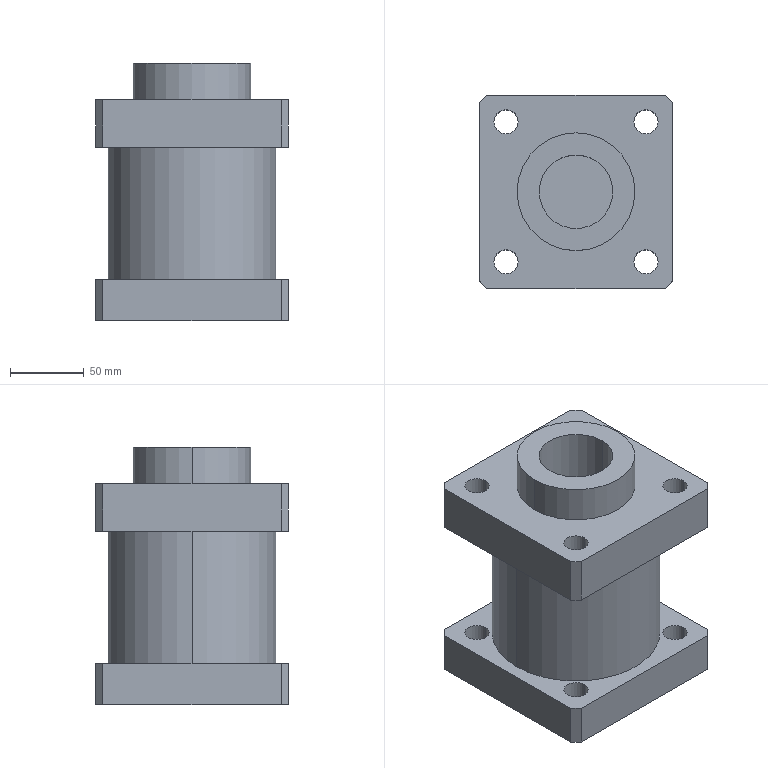Part | SolidWorks | features BaseBody 1 | 1 solid | 55 faces | box 131 x 131 x 175 mm | volume 1197322 mm3 | cylinder 28 | plane 23 | cone 4 | commonest cylinder face diameters 16.5 x16 11.8 x4 50 x2 80 x2 100 x2 114 x2